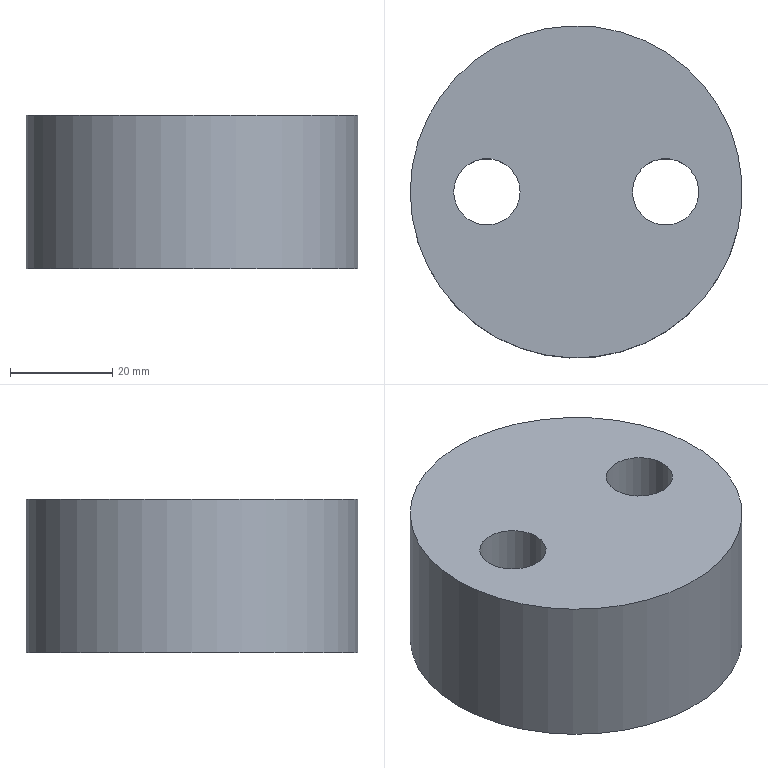Part | NX | features solid 2 | 1 solid | 9 faces | box 65 x 65 x 30 mm | volume 86142 mm3 | cylinder 5 | plane 4 | commonest cylinder face diameters 13 x2 20 x2 65 x1
STEP:
#1=CARTESIAN_POINT('',(1062.5,-930.,125.));
#2=VERTEX_POINT('',#1);
#3=CARTESIAN_POINT('',(1095.,-930.,125.));
#4=DIRECTION('',(0.,0.,-1.));
#5=DIRECTION('',(-1.,0.,0.));
#6=AXIS2_PLACEMENT_3D('',#3,#4,#5);
#7=CIRCLE('',#6,32.5);
#8=EDGE_CURVE('',#2,#2,#7,.T.);
#9=ORIENTED_EDGE('',*,*,#8,.T.);
#10=EDGE_LOOP('',(#9));
#11=FACE_BOUND('',#10,.T.);
#12=CARTESIAN_POINT('',(1062.5,-930.,95.));
#13=VERTEX_POINT('',#12);
#14=CARTESIAN_POINT('',(1095.,-930.,95.));
#15=DIRECTION('',(0.,0.,-1.));
#16=DIRECTION('',(-1.,0.,0.));
#17=AXIS2_PLACEMENT_3D('',#14,#15,#16);
#18=CIRCLE('',#17,32.5);
#19=EDGE_CURVE('',#13,#13,#18,.T.);
#20=ORIENTED_EDGE('',*,*,#19,.F.);
#21=EDGE_LOOP('',(#20));
#22=FACE_BOUND('',#21,.T.);
#23=CARTESIAN_POINT('',(1095.,-930.,115.));
#24=DIRECTION('',(0.,0.,-1.));
#25=DIRECTION('',(1.,0.,0.));
#26=AXIS2_PLACEMENT_3D('',#23,#24,#25);
#27=CYLINDRICAL_SURFACE('',#26,32.5);
#28=ADVANCED_FACE('',(#11,#22),#27,.T.);
#29=CARTESIAN_POINT('',(1071.,-930.,125.));
#30=VERTEX_POINT('',#29);
#31=CARTESIAN_POINT('',(1077.5,-930.,125.));
#32=DIRECTION('',(0.,0.,-1.));
#33=DIRECTION('',(-1.,0.,0.));
#34=AXIS2_PLACEMENT_3D('',#31,#32,#33);
#35=CIRCLE('',#34,6.5);
#36=EDGE_CURVE('',#30,#30,#35,.T.);
#37=ORIENTED_EDGE('',*,*,#36,.T.);
#38=EDGE_LOOP('',(#37));
#39=FACE_BOUND('',#38,.T.);
#40=CARTESIAN_POINT('',(1106.,-930.,125.));
#41=VERTEX_POINT('',#40);
#42=CARTESIAN_POINT('',(1112.5,-930.,125.));
#43=DIRECTION('',(0.,0.,-1.));
#44=DIRECTION('',(-1.,0.,0.));
#45=AXIS2_PLACEMENT_3D('',#42,#43,#44);
#46=CIRCLE('',#45,6.5);
#47=EDGE_CURVE('',#41,#41,#46,.T.);
#48=ORIENTED_EDGE('',*,*,#47,.T.);
#49=EDGE_LOOP('',(#48));
#50=FACE_BOUND('',#49,.T.);
#51=ORIENTED_EDGE('',*,*,#8,.F.);
#52=EDGE_LOOP('',(#51));
#53=FACE_BOUND('',#52,.T.);
#54=CARTESIAN_POINT('',(1095.,-930.,125.));
#55=DIRECTION('',(0.,0.,1.));
#56=DIRECTION('',(-1.,0.,0.));
#57=AXIS2_PLACEMENT_3D('',#54,#55,#56);
#58=PLANE('',#57);
#59=ADVANCED_FACE('',(#39,#50,#53),#58,.T.);
#60=CARTESIAN_POINT('',(1067.5,-930.,95.));
#61=VERTEX_POINT('',#60);
#62=CARTESIAN_POINT('',(1077.5,-930.,95.));
#63=DIRECTION('',(0.,0.,-1.));
#64=DIRECTION('',(-1.,0.,0.));
#65=AXIS2_PLACEMENT_3D('',#62,#63,#64);
#66=CIRCLE('',#65,10.);
#67=EDGE_CURVE('',#61,#61,#66,.T.);
#68=ORIENTED_EDGE('',*,*,#67,.F.);
#69=EDGE_LOOP('',(#68));
#70=FACE_BOUND('',#69,.T.);
#71=CARTESIAN_POINT('',(1102.5,-930.,95.));
#72=VERTEX_POINT('',#71);
#73=CARTESIAN_POINT('',(1112.5,-930.,95.));
#74=DIRECTION('',(0.,0.,-1.));
#75=DIRECTION('',(-1.,0.,0.));
#76=AXIS2_PLACEMENT_3D('',#73,#74,#75);
#77=CIRCLE('',#76,10.);
#78=EDGE_CURVE('',#72,#72,#77,.T.);
#79=ORIENTED_EDGE('',*,*,#78,.F.);
#80=EDGE_LOOP('',(#79));
#81=FACE_BOUND('',#80,.T.);
#82=ORIENTED_EDGE('',*,*,#19,.T.);
#83=EDGE_LOOP('',(#82));
#84=FACE_BOUND('',#83,.T.);
#85=CARTESIAN_POINT('',(1095.,-930.,95.));
#86=DIRECTION('',(0.,0.,1.));
#87=DIRECTION('',(-1.,0.,0.));
#88=AXIS2_PLACEMENT_3D('',#85,#86,#87);
#89=PLANE('',#88);
#90=ADVANCED_FACE('',(#70,#81,#84),#89,.F.);
#91=ORIENTED_EDGE('',*,*,#47,.F.);
#92=EDGE_LOOP('',(#91));
#93=FACE_BOUND('',#92,.T.);
#94=CARTESIAN_POINT('',(1106.,-930.,110.));
#95=VERTEX_POINT('',#94);
#96=CARTESIAN_POINT('',(1112.5,-930.,110.));
#97=DIRECTION('',(0.,0.,-1.));
#98=DIRECTION('',(-1.,0.,0.));
#99=AXIS2_PLACEMENT_3D('',#96,#97,#98);
#100=CIRCLE('',#99,6.5);
#101=EDGE_CURVE('',#95,#95,#100,.T.);
#102=ORIENTED_EDGE('',*,*,#101,.T.);
#103=EDGE_LOOP('',(#102));
#104=FACE_BOUND('',#103,.T.);
#105=CARTESIAN_POINT('',(1112.5,-930.,125.));
#106=DIRECTION('',(0.,0.,1.));
#107=DIRECTION('',(-1.,0.,0.));
#108=AXIS2_PLACEMENT_3D('',#105,#106,#107);
#109=CYLINDRICAL_SURFACE('',#108,6.5);
#110=ADVANCED_FACE('',(#93,#104),#109,.F.);
#111=ORIENTED_EDGE('',*,*,#101,.F.);
#112=EDGE_LOOP('',(#111));
#113=FACE_BOUND('',#112,.T.);
#114=CARTESIAN_POINT('',(1102.5,-930.,110.));
#115=VERTEX_POINT('',#114);
#116=CARTESIAN_POINT('',(1112.5,-930.,110.));
#117=DIRECTION('',(0.,0.,-1.));
#118=DIRECTION('',(-1.,0.,0.));
#119=AXIS2_PLACEMENT_3D('',#116,#117,#118);
#120=CIRCLE('',#119,10.);
#121=EDGE_CURVE('',#115,#115,#120,.T.);
#122=ORIENTED_EDGE('',*,*,#121,.T.);
#123=EDGE_LOOP('',(#122));
#124=FACE_BOUND('',#123,.T.);
#125=CARTESIAN_POINT('',(1112.5,-930.,110.));
#126=DIRECTION('',(0.,0.,1.));
#127=DIRECTION('',(-1.,0.,0.));
#128=AXIS2_PLACEMENT_3D('',#125,#126,#127);
#129=PLANE('',#128);
#130=ADVANCED_FACE('',(#113,#124),#129,.F.);
#131=ORIENTED_EDGE('',*,*,#121,.F.);
#132=EDGE_LOOP('',(#131));
#133=FACE_BOUND('',#132,.T.);
#134=ORIENTED_EDGE('',*,*,#78,.T.);
#135=EDGE_LOOP('',(#134));
#136=FACE_BOUND('',#135,.T.);
#137=CARTESIAN_POINT('',(1112.5,-930.,95.));
#138=DIRECTION('',(0.,0.,1.));
#139=DIRECTION('',(-1.,0.,0.));
#140=AXIS2_PLACEMENT_3D('',#137,#138,#139);
#141=CYLINDRICAL_SURFACE('',#140,10.);
#142=ADVANCED_FACE('',(#133,#136),#141,.F.);
#143=ORIENTED_EDGE('',*,*,#36,.F.);
#144=EDGE_LOOP('',(#143));
#145=FACE_BOUND('',#144,.T.);
#146=CARTESIAN_POINT('',(1071.,-930.,110.));
#147=VERTEX_POINT('',#146);
#148=CARTESIAN_POINT('',(1077.5,-930.,110.));
#149=DIRECTION('',(0.,0.,-1.));
#150=DIRECTION('',(-1.,0.,0.));
#151=AXIS2_PLACEMENT_3D('',#148,#149,#150);
#152=CIRCLE('',#151,6.5);
#153=EDGE_CURVE('',#147,#147,#152,.T.);
#154=ORIENTED_EDGE('',*,*,#153,.T.);
#155=EDGE_LOOP('',(#154));
#156=FACE_BOUND('',#155,.T.);
#157=CARTESIAN_POINT('',(1077.5,-930.,125.));
#158=DIRECTION('',(0.,0.,1.));
#159=DIRECTION('',(-1.,0.,0.));
#160=AXIS2_PLACEMENT_3D('',#157,#158,#159);
#161=CYLINDRICAL_SURFACE('',#160,6.5);
#162=ADVANCED_FACE('',(#145,#156),#161,.F.);
#163=ORIENTED_EDGE('',*,*,#153,.F.);
#164=EDGE_LOOP('',(#163));
#165=FACE_BOUND('',#164,.T.);
#166=CARTESIAN_POINT('',(1067.5,-930.,110.));
#167=VERTEX_POINT('',#166);
#168=CARTESIAN_POINT('',(1077.5,-930.,110.));
#169=DIRECTION('',(0.,0.,-1.));
#170=DIRECTION('',(-1.,0.,0.));
#171=AXIS2_PLACEMENT_3D('',#168,#169,#170);
#172=CIRCLE('',#171,10.);
#173=EDGE_CURVE('',#167,#167,#172,.T.);
#174=ORIENTED_EDGE('',*,*,#173,.T.);
#175=EDGE_LOOP('',(#174));
#176=FACE_BOUND('',#175,.T.);
#177=CARTESIAN_POINT('',(1077.5,-930.,110.));
#178=DIRECTION('',(0.,0.,1.));
#179=DIRECTION('',(-1.,0.,0.));
#180=AXIS2_PLACEMENT_3D('',#177,#178,#179);
#181=PLANE('',#180);
#182=ADVANCED_FACE('',(#165,#176),#181,.F.);
#183=ORIENTED_EDGE('',*,*,#173,.F.);
#184=EDGE_LOOP('',(#183));
#185=FACE_BOUND('',#184,.T.);
#186=ORIENTED_EDGE('',*,*,#67,.T.);
#187=EDGE_LOOP('',(#186));
#188=FACE_BOUND('',#187,.T.);
#189=CARTESIAN_POINT('',(1077.5,-930.,95.));
#190=DIRECTION('',(0.,0.,1.));
#191=DIRECTION('',(-1.,0.,0.));
#192=AXIS2_PLACEMENT_3D('',#189,#190,#191);
#193=CYLINDRICAL_SURFACE('',#192,10.);
#194=ADVANCED_FACE('',(#185,#188),#193,.F.);
#195=CLOSED_SHELL('',(#28,#59,#90,#110,#130,#142,#162,#182,#194));
#196=MANIFOLD_SOLID_BREP('',#195);
#197=(LENGTH_UNIT()NAMED_UNIT(*)SI_UNIT(.MILLI.,.METRE.));
#198=UNCERTAINTY_MEASURE_WITH_UNIT(LENGTH_MEASURE(0.00001),#197,'','');
#199=(NAMED_UNIT(*)PLANE_ANGLE_UNIT()SI_UNIT($,.RADIAN.));
#200=(NAMED_UNIT(*)SI_UNIT($,.STERADIAN.)SOLID_ANGLE_UNIT());
#201=(GEOMETRIC_REPRESENTATION_CONTEXT(3)GLOBAL_UNCERTAINTY_ASSIGNED_CONTEXT((#198))GLOBAL_UNIT_ASSIGNED_CONTEXT((#197,#199,#200))REPRESENTATION_CONTEXT('',''));
#202=ADVANCED_BREP_SHAPE_REPRESENTATION('',(#196),#201);